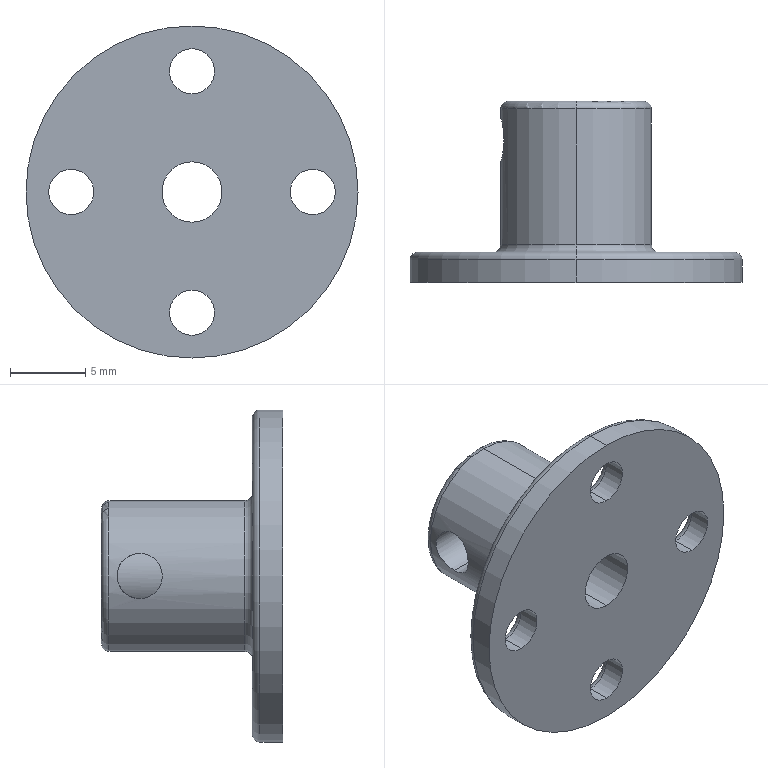Part | STEP file | Flange coupling 4 | 1 solid | 34 faces | box 22 x 12 x 22 mm | volume 1314 mm3 | cylinder 17 | torus 14 | plane 3 | commonest cylinder face diameters 3 x10 4 x2 10 x2 22 x2 5 x1